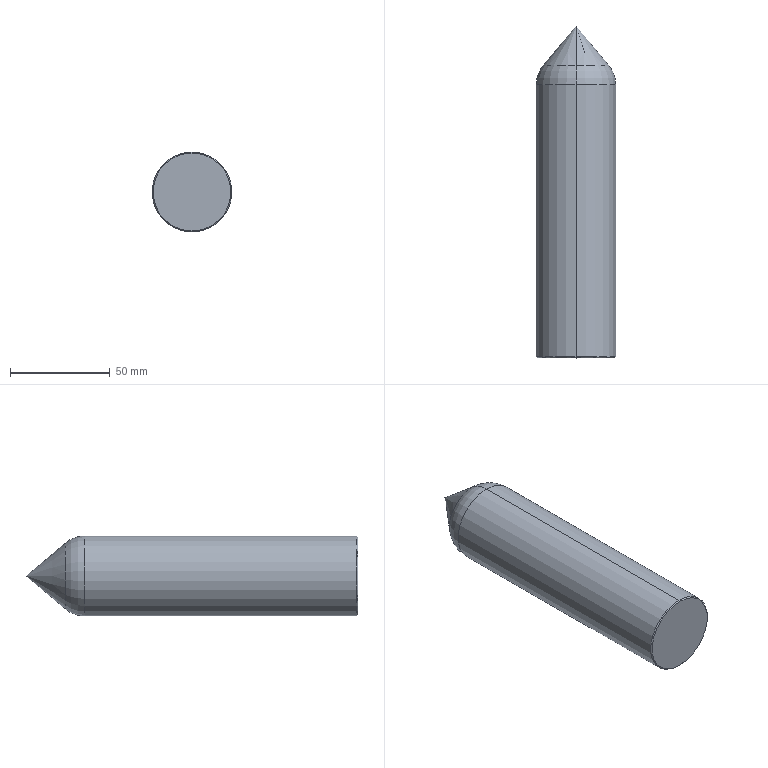Part | SolidWorks | features Chamfer 1, Fillet 1, Revolution 1 | 1 solid | 9 faces | box 40 x 166 x 40 mm | volume 188212 mm3 | cone 4 | torus 2 | cylinder 2 | plane 1 | commonest cylinder face diameters 40 x2
STEP:
#1=CARTESIAN_POINT('',(0.,-166.,-19.5));
#2=VERTEX_POINT('',#1);
#3=CARTESIAN_POINT('',(0.,-166.,19.5));
#4=VERTEX_POINT('',#3);
#5=CARTESIAN_POINT('',(0.,-166.,0.));
#6=DIRECTION('',(0.,-1.,0.));
#7=DIRECTION('',(0.,0.,1.));
#8=AXIS2_PLACEMENT_3D('',#5,#6,#7);
#9=CIRCLE('',#8,19.5);
#10=EDGE_CURVE('',#2,#4,#9,.T.);
#11=ORIENTED_EDGE('',*,*,#10,.F.);
#12=CARTESIAN_POINT('',(0.,-165.5,-20.));
#13=VERTEX_POINT('',#12);
#14=CARTESIAN_POINT('',(0.,-166.,-19.5));
#15=DIRECTION('',(0.,0.7071,-0.7071));
#16=VECTOR('',#15,1000.);
#17=LINE('',#14,#16);
#18=EDGE_CURVE('',#2,#13,#17,.T.);
#19=ORIENTED_EDGE('',*,*,#18,.T.);
#20=CARTESIAN_POINT('',(0.,-165.5,20.));
#21=VERTEX_POINT('',#20);
#22=CARTESIAN_POINT('',(0.,-165.5,0.));
#23=DIRECTION('',(0.,1.,0.));
#24=DIRECTION('',(0.,0.,1.));
#25=AXIS2_PLACEMENT_3D('',#22,#23,#24);
#26=CIRCLE('',#25,20.);
#27=EDGE_CURVE('',#21,#13,#26,.T.);
#28=ORIENTED_EDGE('',*,*,#27,.F.);
#29=CARTESIAN_POINT('',(0.,-166.,19.5));
#30=DIRECTION('',(0.,0.7071,0.7071));
#31=VECTOR('',#30,1000.);
#32=LINE('',#29,#31);
#33=EDGE_CURVE('',#4,#21,#32,.T.);
#34=ORIENTED_EDGE('',*,*,#33,.F.);
#35=EDGE_LOOP('',(#11,#19,#28,#34));
#36=FACE_OUTER_BOUND('',#35,.T.);
#37=CARTESIAN_POINT('',(0.,-166.,0.));
#38=DIRECTION('',(0.,1.,0.));
#39=DIRECTION('',(0.,0.,1.));
#40=AXIS2_PLACEMENT_3D('',#37,#38,#39);
#41=CONICAL_SURFACE('',#40,19.5,0.7854);
#42=ADVANCED_FACE('',(#36),#41,.T.);
#43=CARTESIAN_POINT('',(0.,-29.295,-20.));
#44=VERTEX_POINT('',#43);
#45=CARTESIAN_POINT('',(0.,-29.295,20.));
#46=VERTEX_POINT('',#45);
#47=CARTESIAN_POINT('',(0.,-29.295,0.));
#48=DIRECTION('',(0.,-1.,0.));
#49=DIRECTION('',(0.,0.,1.));
#50=AXIS2_PLACEMENT_3D('',#47,#48,#49);
#51=CIRCLE('',#50,20.);
#52=EDGE_CURVE('',#44,#46,#51,.T.);
#53=ORIENTED_EDGE('',*,*,#52,.F.);
#54=CARTESIAN_POINT('',(0.,-19.653,-16.491));
#55=VERTEX_POINT('',#54);
#56=CARTESIAN_POINT('',(0.,-29.295,-5.));
#57=DIRECTION('',(1.,0.,0.));
#58=DIRECTION('',(0.,0.,-1.));
#59=AXIS2_PLACEMENT_3D('',#56,#57,#58);
#60=CIRCLE('',#59,15.);
#61=EDGE_CURVE('',#44,#55,#60,.T.);
#62=ORIENTED_EDGE('',*,*,#61,.T.);
#63=CARTESIAN_POINT('',(0.,-19.653,16.491));
#64=VERTEX_POINT('',#63);
#65=CARTESIAN_POINT('',(0.,-19.653,0.));
#66=DIRECTION('',(0.,1.,0.));
#67=DIRECTION('',(0.,0.,1.));
#68=AXIS2_PLACEMENT_3D('',#65,#66,#67);
#69=CIRCLE('',#68,16.491);
#70=EDGE_CURVE('',#64,#55,#69,.T.);
#71=ORIENTED_EDGE('',*,*,#70,.F.);
#72=CARTESIAN_POINT('',(0.,-29.295,5.));
#73=DIRECTION('',(-1.,0.,0.));
#74=DIRECTION('',(0.,0.,1.));
#75=AXIS2_PLACEMENT_3D('',#72,#73,#74);
#76=CIRCLE('',#75,15.);
#77=EDGE_CURVE('',#46,#64,#76,.T.);
#78=ORIENTED_EDGE('',*,*,#77,.F.);
#79=EDGE_LOOP('',(#53,#62,#71,#78));
#80=FACE_OUTER_BOUND('',#79,.T.);
#81=CARTESIAN_POINT('',(0.,-29.295,0.));
#82=DIRECTION('',(0.,1.,0.));
#83=DIRECTION('',(0.,0.,1.));
#84=AXIS2_PLACEMENT_3D('',#81,#82,#83);
#85=TOROIDAL_SURFACE('',#84,5.,15.);
#86=ADVANCED_FACE('',(#80),#85,.T.);
#87=CARTESIAN_POINT('',(0.,0.,0.));
#88=VERTEX_POINT('',#87);
#89=CARTESIAN_POINT('',(0.,0.,0.));
#90=DIRECTION('',(0.,-0.766,-0.6428));
#91=VECTOR('',#90,1000.);
#92=LINE('',#89,#91);
#93=EDGE_CURVE('',#88,#55,#92,.T.);
#94=ORIENTED_EDGE('',*,*,#93,.F.);
#95=CARTESIAN_POINT('',(0.,0.,0.));
#96=DIRECTION('',(0.,-0.766,0.6428));
#97=VECTOR('',#96,1000.);
#98=LINE('',#95,#97);
#99=EDGE_CURVE('',#88,#64,#98,.T.);
#100=ORIENTED_EDGE('',*,*,#99,.T.);
#101=ORIENTED_EDGE('',*,*,#70,.T.);
#102=EDGE_LOOP('',(#94,#100,#101));
#103=FACE_OUTER_BOUND('',#102,.T.);
#104=CARTESIAN_POINT('',(0.,-1000.,0.));
#105=DIRECTION('',(0.,-1.,0.));
#106=DIRECTION('',(0.,0.,-1.));
#107=AXIS2_PLACEMENT_3D('',#104,#105,#106);
#108=CONICAL_SURFACE('',#107,839.1,0.6981);
#109=ADVANCED_FACE('',(#103),#108,.T.);
#110=ORIENTED_EDGE('',*,*,#52,.T.);
#111=CARTESIAN_POINT('',(0.,-166.,20.));
#112=DIRECTION('',(0.,-1.,0.));
#113=VECTOR('',#112,1000.);
#114=LINE('',#111,#113);
#115=EDGE_CURVE('',#46,#21,#114,.T.);
#116=ORIENTED_EDGE('',*,*,#115,.T.);
#117=ORIENTED_EDGE('',*,*,#27,.T.);
#118=CARTESIAN_POINT('',(0.,-166.,-20.));
#119=DIRECTION('',(0.,-1.,0.));
#120=VECTOR('',#119,1000.);
#121=LINE('',#118,#120);
#122=EDGE_CURVE('',#44,#13,#121,.T.);
#123=ORIENTED_EDGE('',*,*,#122,.F.);
#124=EDGE_LOOP('',(#110,#116,#117,#123));
#125=FACE_OUTER_BOUND('',#124,.T.);
#126=CARTESIAN_POINT('',(0.,-166.,0.));
#127=DIRECTION('',(0.,-1.,0.));
#128=DIRECTION('',(0.,0.,-1.));
#129=AXIS2_PLACEMENT_3D('',#126,#127,#128);
#130=CYLINDRICAL_SURFACE('',#129,20.);
#131=ADVANCED_FACE('',(#125),#130,.T.);
#132=CARTESIAN_POINT('',(0.,-166.,0.));
#133=DIRECTION('',(0.,-1.,0.));
#134=DIRECTION('',(0.,0.,1.));
#135=AXIS2_PLACEMENT_3D('',#132,#133,#134);
#136=CIRCLE('',#135,19.5);
#137=EDGE_CURVE('',#4,#2,#136,.T.);
#138=ORIENTED_EDGE('',*,*,#137,.T.);
#139=ORIENTED_EDGE('',*,*,#10,.T.);
#140=EDGE_LOOP('',(#138,#139));
#141=FACE_OUTER_BOUND('',#140,.T.);
#142=CARTESIAN_POINT('',(-20.,-166.,0.));
#143=DIRECTION('',(0.,1.,0.));
#144=DIRECTION('',(0.,0.,1.));
#145=AXIS2_PLACEMENT_3D('',#142,#143,#144);
#146=PLANE('',#145);
#147=ADVANCED_FACE('',(#141),#146,.F.);
#148=ORIENTED_EDGE('',*,*,#115,.F.);
#149=CARTESIAN_POINT('',(0.,-29.295,0.));
#150=DIRECTION('',(0.,-1.,0.));
#151=DIRECTION('',(0.,0.,1.));
#152=AXIS2_PLACEMENT_3D('',#149,#150,#151);
#153=CIRCLE('',#152,20.);
#154=EDGE_CURVE('',#46,#44,#153,.T.);
#155=ORIENTED_EDGE('',*,*,#154,.T.);
#156=ORIENTED_EDGE('',*,*,#122,.T.);
#157=CARTESIAN_POINT('',(0.,-165.5,0.));
#158=DIRECTION('',(0.,1.,0.));
#159=DIRECTION('',(0.,0.,1.));
#160=AXIS2_PLACEMENT_3D('',#157,#158,#159);
#161=CIRCLE('',#160,20.);
#162=EDGE_CURVE('',#13,#21,#161,.T.);
#163=ORIENTED_EDGE('',*,*,#162,.T.);
#164=EDGE_LOOP('',(#148,#155,#156,#163));
#165=FACE_OUTER_BOUND('',#164,.T.);
#166=CARTESIAN_POINT('',(0.,-166.,0.));
#167=DIRECTION('',(0.,-1.,0.));
#168=DIRECTION('',(0.,0.,-1.));
#169=AXIS2_PLACEMENT_3D('',#166,#167,#168);
#170=CYLINDRICAL_SURFACE('',#169,20.);
#171=ADVANCED_FACE('',(#165),#170,.T.);
#172=ORIENTED_EDGE('',*,*,#99,.F.);
#173=ORIENTED_EDGE('',*,*,#93,.T.);
#174=CARTESIAN_POINT('',(0.,-19.653,0.));
#175=DIRECTION('',(0.,1.,0.));
#176=DIRECTION('',(0.,0.,1.));
#177=AXIS2_PLACEMENT_3D('',#174,#175,#176);
#178=CIRCLE('',#177,16.491);
#179=EDGE_CURVE('',#55,#64,#178,.T.);
#180=ORIENTED_EDGE('',*,*,#179,.T.);
#181=EDGE_LOOP('',(#172,#173,#180));
#182=FACE_OUTER_BOUND('',#181,.T.);
#183=CARTESIAN_POINT('',(0.,-1000.,0.));
#184=DIRECTION('',(0.,-1.,0.));
#185=DIRECTION('',(0.,0.,-1.));
#186=AXIS2_PLACEMENT_3D('',#183,#184,#185);
#187=CONICAL_SURFACE('',#186,839.1,0.6981);
#188=ADVANCED_FACE('',(#182),#187,.T.);
#189=ORIENTED_EDGE('',*,*,#61,.F.);
#190=ORIENTED_EDGE('',*,*,#154,.F.);
#191=ORIENTED_EDGE('',*,*,#77,.T.);
#192=ORIENTED_EDGE('',*,*,#179,.F.);
#193=EDGE_LOOP('',(#189,#190,#191,#192));
#194=FACE_OUTER_BOUND('',#193,.T.);
#195=CARTESIAN_POINT('',(0.,-29.295,0.));
#196=DIRECTION('',(0.,1.,0.));
#197=DIRECTION('',(0.,0.,1.));
#198=AXIS2_PLACEMENT_3D('',#195,#196,#197);
#199=TOROIDAL_SURFACE('',#198,5.,15.);
#200=ADVANCED_FACE('',(#194),#199,.T.);
#201=ORIENTED_EDGE('',*,*,#18,.F.);
#202=ORIENTED_EDGE('',*,*,#137,.F.);
#203=ORIENTED_EDGE('',*,*,#33,.T.);
#204=ORIENTED_EDGE('',*,*,#162,.F.);
#205=EDGE_LOOP('',(#201,#202,#203,#204));
#206=FACE_OUTER_BOUND('',#205,.T.);
#207=CARTESIAN_POINT('',(0.,-166.,0.));
#208=DIRECTION('',(0.,1.,0.));
#209=DIRECTION('',(0.,0.,1.));
#210=AXIS2_PLACEMENT_3D('',#207,#208,#209);
#211=CONICAL_SURFACE('',#210,19.5,0.7854);
#212=ADVANCED_FACE('',(#206),#211,.T.);
#213=CLOSED_SHELL('',(#42,#86,#109,#131,#147,#171,#188,#200,#212));
#214=MANIFOLD_SOLID_BREP('',#213);
#215=CARTESIAN_POINT('',(0.,0.,0.));
#216=DIRECTION('',(0.,0.,1.));
#217=DIRECTION('',(1.,0.,0.));
#218=AXIS2_PLACEMENT_3D('',#215,#216,#217);
#219=(LENGTH_UNIT()NAMED_UNIT(*)SI_UNIT(.MILLI.,.METRE.));
#220=UNCERTAINTY_MEASURE_WITH_UNIT(LENGTH_MEASURE(0.00001),#219,'','');
#221=(NAMED_UNIT(*)PLANE_ANGLE_UNIT()SI_UNIT($,.RADIAN.));
#222=(NAMED_UNIT(*)SI_UNIT($,.STERADIAN.)SOLID_ANGLE_UNIT());
#223=(GEOMETRIC_REPRESENTATION_CONTEXT(3)GLOBAL_UNCERTAINTY_ASSIGNED_CONTEXT((#220))GLOBAL_UNIT_ASSIGNED_CONTEXT((#219,#221,#222))REPRESENTATION_CONTEXT('',''));
#224=ADVANCED_BREP_SHAPE_REPRESENTATION('',(#214,#218),#223);